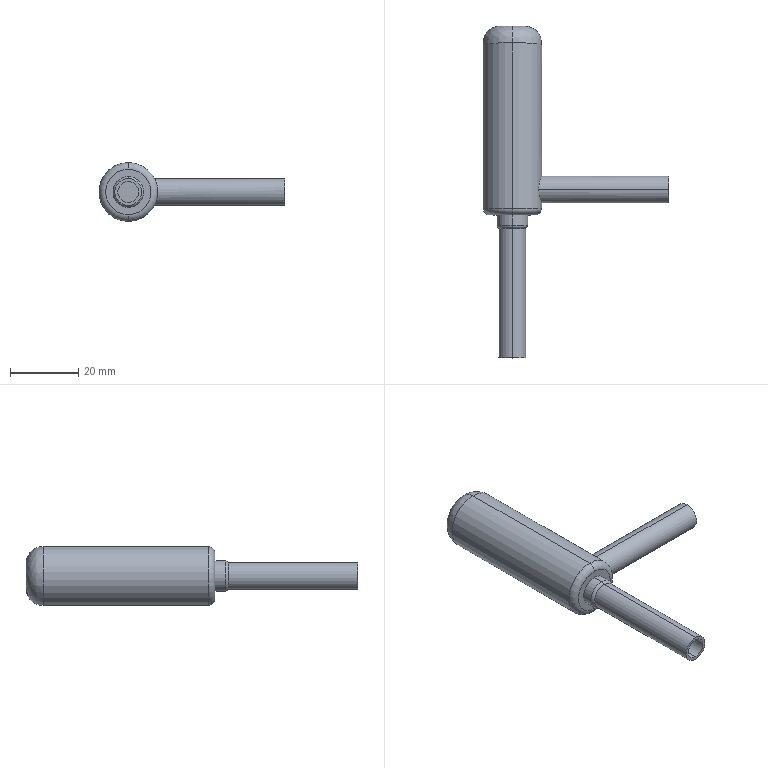Part | STEP file | cooling electronic expansion valve | 1 solid | 25 faces | box 54.65 x 97.5 x 17.3 mm | volume 14688 mm3 | cylinder 12 | plane 7 | torus 4 | other 2 | commonest cylinder face diameters 6.14 x4 7.9 x4 9 x2 17.3 x2